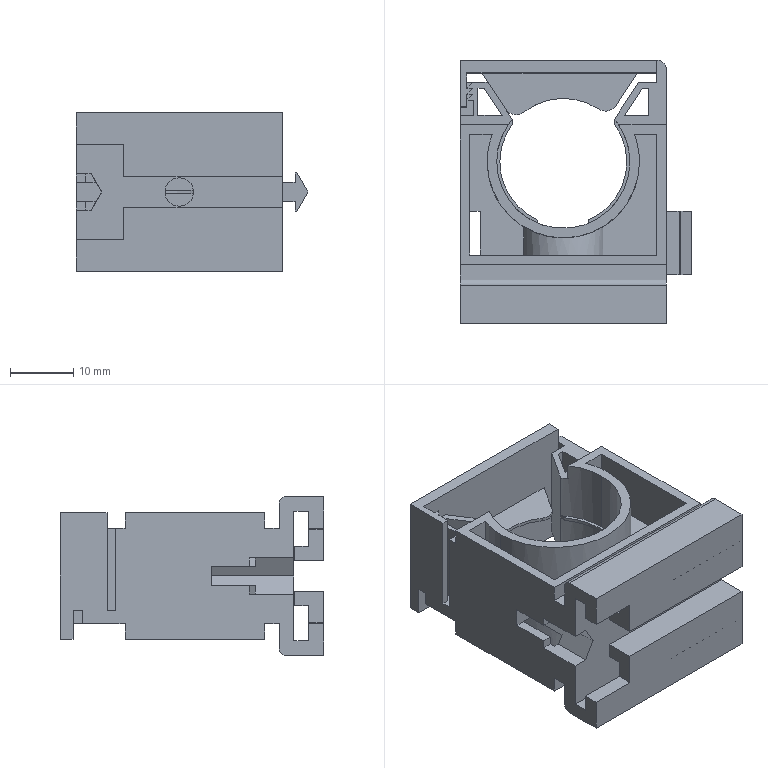Part | STEP file | 00192289_KLEMMSCHELLE_MKRS-16.5-B.1 | 1 solid | 148 faces | box 36.5 x 41.5 x 25 mm | volume 11692 mm3 | plane 120 | cylinder 28 | commonest cylinder face diameters 21 x6 24 x6 20 x4 12.8 x3 2 x2 4 x2